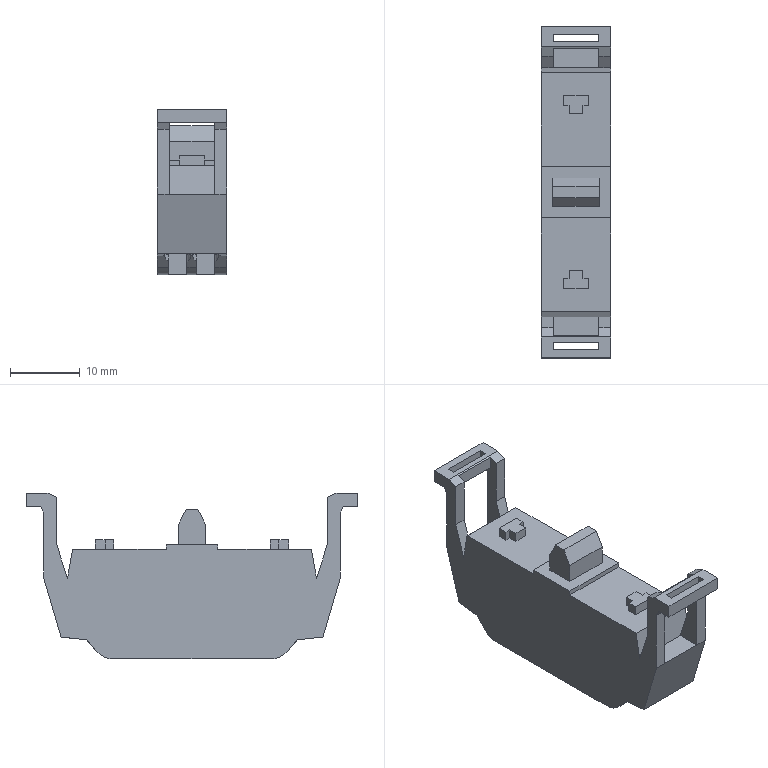Part | STEP file | A22NZ_S_P1[]N | 1 solid | 145 faces | box 9.9 x 47.6 x 23.8 mm | volume 5482 mm3 | plane 127 | cylinder 18 | commonest cylinder face diameters 2.8 x6 4.2 x6 6.4 x6